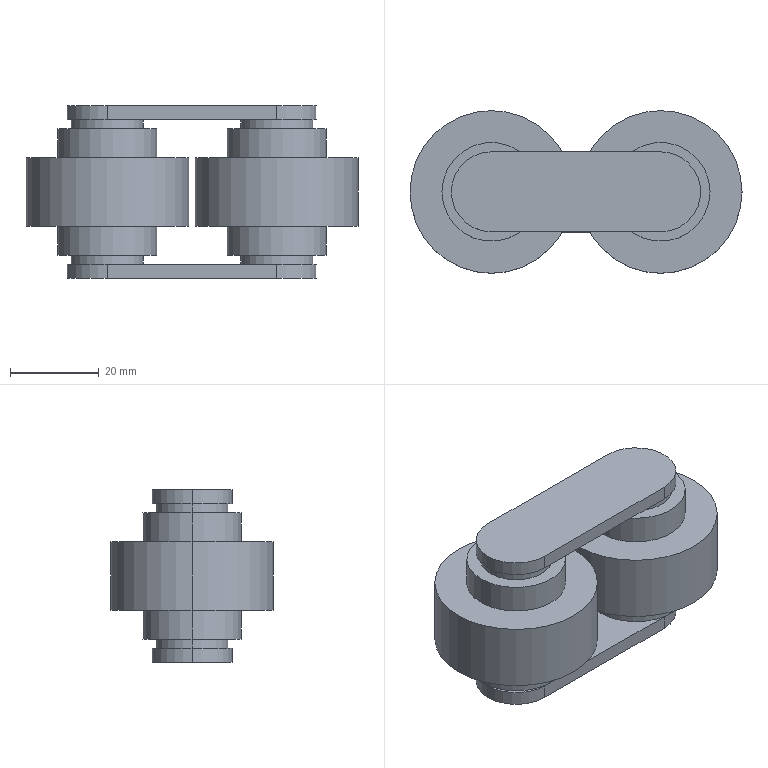Part | STEP file | PN_0022_default | 1 solid | 42 faces | box 74.7 x 36.6 x 38.9 mm | volume 50379 mm3 | cylinder 26 | plane 16 | commonest cylinder face diameters 16.23 x8 22.23 x8 18 x6 36.6 x4